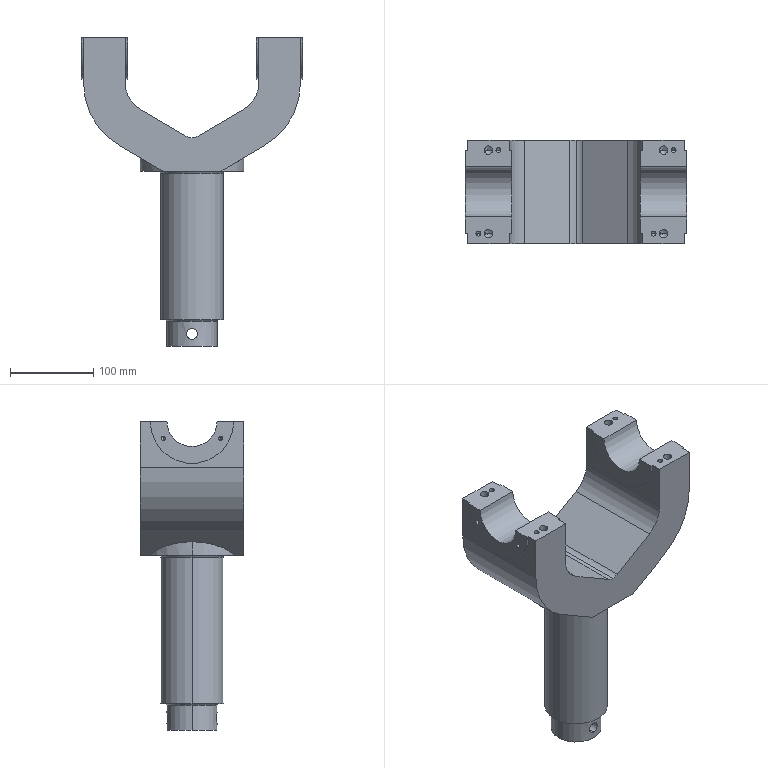Part | SolidWorks | features ICE 7, HoleWzd 3, Chamfer 1, Extrusion 1, Fillet 1, MirrorPattern 1 | 1 solid | 94 faces | box 265 x 124 x 370 mm | volume 3221545 mm3 | cylinder 45 | cone 26 | plane 21 | torus 2 | commonest cylinder face diameters 5 x8 6 x8 10.2 x8 60 x4 100 x4 124 x3